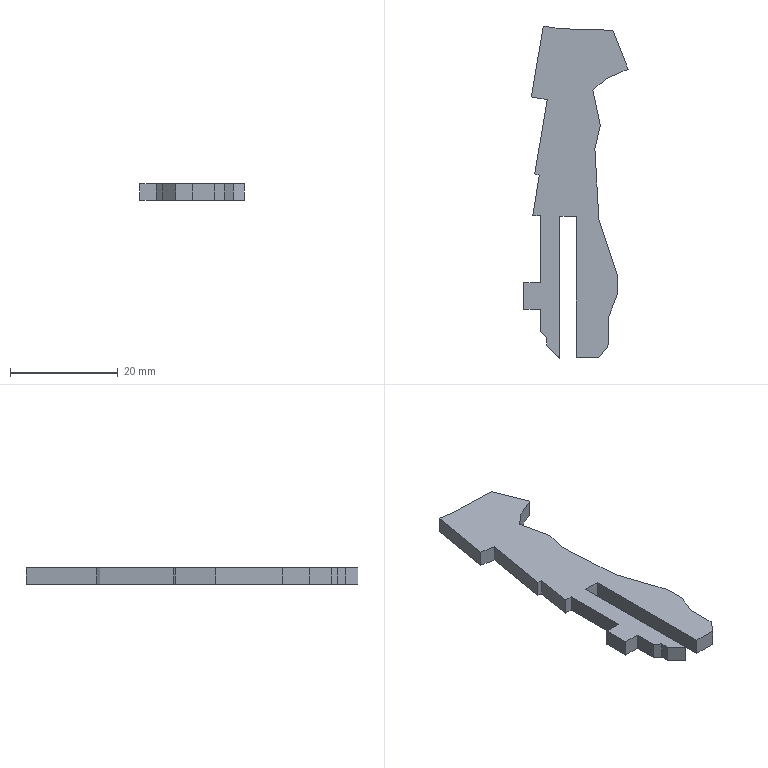Part | SolidWorks | features BaseBody 1 | 1 solid | 33 faces | box 19.346 x 61.524 x 3 mm | volume 2044 mm3 | spline 18 | plane 15
STEP:
#1=CARTESIAN_POINT('',(30.02,-31.07,-1.5));
#2=VERTEX_POINT('',#1);
#3=CARTESIAN_POINT('',(29.997,-32.532,-1.5));
#4=VERTEX_POINT('',#3);
#5=CARTESIAN_POINT('',(30.02,-31.07,-1.5));
#6=CARTESIAN_POINT('',(30.011,-31.556,-1.5));
#7=CARTESIAN_POINT('',(30.004,-32.045,-1.5));
#8=CARTESIAN_POINT('',(29.997,-32.532,-1.5));
#9=B_SPLINE_CURVE_WITH_KNOTS('',3,(#5,#6,#7,#8),.UNSPECIFIED.,.F.,.F.,(4,4),(0.,0.02857),.UNSPECIFIED.);
#10=EDGE_CURVE('',#2,#4,#9,.T.);
#11=ORIENTED_EDGE('',*,*,#10,.F.);
#12=CARTESIAN_POINT('',(28.815,-30.046,-1.5));
#13=VERTEX_POINT('',#12);
#14=CARTESIAN_POINT('',(28.815,-30.046,-1.5));
#15=CARTESIAN_POINT('',(29.216,-30.385,-1.5));
#16=CARTESIAN_POINT('',(29.619,-30.728,-1.5));
#17=CARTESIAN_POINT('',(30.02,-31.07,-1.5));
#18=B_SPLINE_CURVE_WITH_KNOTS('',3,(#14,#15,#16,#17),.UNSPECIFIED.,.F.,.F.,(4,4),(0.02857,0.05714),.UNSPECIFIED.);
#19=EDGE_CURVE('',#13,#2,#18,.T.);
#20=ORIENTED_EDGE('',*,*,#19,.F.);
#21=CARTESIAN_POINT('',(28.813,-25.837,-1.5));
#22=VERTEX_POINT('',#21);
#23=CARTESIAN_POINT('',(28.815,-30.046,-1.5));
#24=DIRECTION('',(0.0006257,-1.,0.));
#25=VECTOR('',#24,1000.);
#26=LINE('',#23,#25);
#27=EDGE_CURVE('',#22,#13,#26,.T.);
#28=ORIENTED_EDGE('',*,*,#27,.F.);
#29=CARTESIAN_POINT('',(25.744,-25.837,-1.5));
#30=VERTEX_POINT('',#29);
#31=CARTESIAN_POINT('',(28.813,-25.837,-1.5));
#32=DIRECTION('',(1.,0.,0.));
#33=VECTOR('',#32,1000.);
#34=LINE('',#31,#33);
#35=EDGE_CURVE('',#30,#22,#34,.T.);
#36=ORIENTED_EDGE('',*,*,#35,.F.);
#37=CARTESIAN_POINT('',(25.744,-20.948,-1.5));
#38=VERTEX_POINT('',#37);
#39=CARTESIAN_POINT('',(25.744,-20.948,-1.5));
#40=DIRECTION('',(0.,-1.,0.));
#41=VECTOR('',#40,1000.);
#42=LINE('',#39,#41);
#43=EDGE_CURVE('',#38,#30,#42,.T.);
#44=ORIENTED_EDGE('',*,*,#43,.F.);
#45=CARTESIAN_POINT('',(28.815,-20.948,-1.5));
#46=VERTEX_POINT('',#45);
#47=CARTESIAN_POINT('',(28.815,-20.948,-1.5));
#48=DIRECTION('',(-1.,0.,0.));
#49=VECTOR('',#48,1000.);
#50=LINE('',#47,#49);
#51=EDGE_CURVE('',#46,#38,#50,.T.);
#52=ORIENTED_EDGE('',*,*,#51,.F.);
#53=CARTESIAN_POINT('',(28.778,-8.507,-1.5));
#54=VERTEX_POINT('',#53);
#55=CARTESIAN_POINT('',(28.778,-8.507,-1.5));
#56=DIRECTION('',(0.00303,-1.,0.));
#57=VECTOR('',#56,1000.);
#58=LINE('',#55,#57);
#59=EDGE_CURVE('',#54,#46,#58,.T.);
#60=ORIENTED_EDGE('',*,*,#59,.F.);
#61=CARTESIAN_POINT('',(27.416,-8.51,-1.5));
#62=VERTEX_POINT('',#61);
#63=CARTESIAN_POINT('',(27.416,-8.51,-1.5));
#64=DIRECTION('',(1.,0.002423,0.));
#65=VECTOR('',#64,1000.);
#66=LINE('',#63,#65);
#67=EDGE_CURVE('',#62,#54,#66,.T.);
#68=ORIENTED_EDGE('',*,*,#67,.F.);
#69=CARTESIAN_POINT('',(28.599,-0.9958,-1.5));
#70=VERTEX_POINT('',#69);
#71=CARTESIAN_POINT('',(28.599,-0.9958,-1.5));
#72=DIRECTION('',(-0.1555,-0.9878,0.));
#73=VECTOR('',#72,1000.);
#74=LINE('',#71,#73);
#75=EDGE_CURVE('',#70,#62,#74,.T.);
#76=ORIENTED_EDGE('',*,*,#75,.F.);
#77=CARTESIAN_POINT('',(27.774,-0.7876,-1.5));
#78=VERTEX_POINT('',#77);
#79=CARTESIAN_POINT('',(27.774,-0.7876,-1.5));
#80=CARTESIAN_POINT('',(28.05,-0.8589,-1.5));
#81=CARTESIAN_POINT('',(28.599,-0.9958,-1.5));
#82=B_SPLINE_CURVE_WITH_KNOTS('',2,(#79,#80,#81),.UNSPECIFIED.,.F.,.F.,(3,3),(0.3143,0.3429),.UNSPECIFIED.);
#83=EDGE_CURVE('',#78,#70,#82,.T.);
#84=ORIENTED_EDGE('',*,*,#83,.F.);
#85=CARTESIAN_POINT('',(30.092,12.981,-1.5));
#86=VERTEX_POINT('',#85);
#87=CARTESIAN_POINT('',(30.092,12.981,-1.5));
#88=CARTESIAN_POINT('',(29.321,8.39,-1.5));
#89=CARTESIAN_POINT('',(28.549,3.8,-1.5));
#90=CARTESIAN_POINT('',(27.774,-0.7876,-1.5));
#91=B_SPLINE_CURVE_WITH_KNOTS('',3,(#87,#88,#89,#90),.UNSPECIFIED.,.F.,.F.,(4,4),(0.3429,0.3714),.UNSPECIFIED.);
#92=EDGE_CURVE('',#86,#78,#91,.T.);
#93=ORIENTED_EDGE('',*,*,#92,.F.);
#94=CARTESIAN_POINT('',(27.138,13.478,-1.5));
#95=VERTEX_POINT('',#94);
#96=CARTESIAN_POINT('',(30.092,12.981,-1.5));
#97=DIRECTION('',(0.9861,-0.1659,0.));
#98=VECTOR('',#97,1000.);
#99=LINE('',#96,#98);
#100=EDGE_CURVE('',#95,#86,#99,.T.);
#101=ORIENTED_EDGE('',*,*,#100,.F.);
#102=CARTESIAN_POINT('',(29.351,26.625,-1.5));
#103=VERTEX_POINT('',#102);
#104=CARTESIAN_POINT('',(29.351,26.625,-1.5));
#105=CARTESIAN_POINT('',(28.613,22.242,-1.5));
#106=CARTESIAN_POINT('',(27.876,17.86,-1.5));
#107=CARTESIAN_POINT('',(27.138,13.478,-1.5));
#108=B_SPLINE_CURVE_WITH_KNOTS('',3,(#104,#105,#106,#107),.UNSPECIFIED.,.F.,.F.,(4,4),(0.4,0.4286),.UNSPECIFIED.);
#109=EDGE_CURVE('',#103,#95,#108,.T.);
#110=ORIENTED_EDGE('',*,*,#109,.F.);
#111=CARTESIAN_POINT('',(32.305,26.126,-1.5));
#112=VERTEX_POINT('',#111);
#113=CARTESIAN_POINT('',(32.305,26.126,-1.5));
#114=CARTESIAN_POINT('',(31.321,26.292,-1.5));
#115=CARTESIAN_POINT('',(30.333,26.457,-1.5));
#116=CARTESIAN_POINT('',(29.351,26.625,-1.5));
#117=B_SPLINE_CURVE_WITH_KNOTS('',3,(#113,#114,#115,#116),.UNSPECIFIED.,.F.,.F.,(4,4),(0.4286,0.4571),.UNSPECIFIED.);
#118=EDGE_CURVE('',#112,#103,#117,.T.);
#119=ORIENTED_EDGE('',*,*,#118,.F.);
#120=CARTESIAN_POINT('',(42.267,25.835,-1.5));
#121=VERTEX_POINT('',#120);
#122=CARTESIAN_POINT('',(42.267,25.835,-1.5));
#123=CARTESIAN_POINT('',(38.946,25.932,-1.5));
#124=CARTESIAN_POINT('',(35.626,26.029,-1.5));
#125=CARTESIAN_POINT('',(32.305,26.126,-1.5));
#126=B_SPLINE_CURVE_WITH_KNOTS('',3,(#122,#123,#124,#125),.UNSPECIFIED.,.F.,.F.,(4,4),(0.4571,0.4857),.UNSPECIFIED.);
#127=EDGE_CURVE('',#121,#112,#126,.T.);
#128=ORIENTED_EDGE('',*,*,#127,.F.);
#129=CARTESIAN_POINT('',(45.09,18.64,-1.5));
#130=VERTEX_POINT('',#129);
#131=CARTESIAN_POINT('',(45.09,18.64,-1.5));
#132=CARTESIAN_POINT('',(44.147,21.036,-1.5));
#133=CARTESIAN_POINT('',(43.208,23.437,-1.5));
#134=CARTESIAN_POINT('',(42.267,25.835,-1.5));
#135=B_SPLINE_CURVE_WITH_KNOTS('',3,(#131,#132,#133,#134),.UNSPECIFIED.,.F.,.F.,(4,4),(0.4857,0.5143),.UNSPECIFIED.);
#136=EDGE_CURVE('',#130,#121,#135,.T.);
#137=ORIENTED_EDGE('',*,*,#136,.F.);
#138=CARTESIAN_POINT('',(41.02,16.861,-1.5));
#139=VERTEX_POINT('',#138);
#140=CARTESIAN_POINT('',(41.02,16.861,-1.5));
#141=CARTESIAN_POINT('',(42.375,17.453,-1.5));
#142=CARTESIAN_POINT('',(43.731,18.045,-1.5));
#143=CARTESIAN_POINT('',(45.09,18.64,-1.5));
#144=B_SPLINE_CURVE_WITH_KNOTS('',3,(#140,#141,#142,#143),.UNSPECIFIED.,.F.,.F.,(4,4),(0.5143,0.5429),.UNSPECIFIED.);
#145=EDGE_CURVE('',#139,#130,#144,.T.);
#146=ORIENTED_EDGE('',*,*,#145,.F.);
#147=CARTESIAN_POINT('',(38.537,14.762,-1.5));
#148=VERTEX_POINT('',#147);
#149=CARTESIAN_POINT('',(38.537,14.762,-1.5));
#150=CARTESIAN_POINT('',(39.365,15.462,-1.5));
#151=CARTESIAN_POINT('',(40.192,16.16,-1.5));
#152=CARTESIAN_POINT('',(41.02,16.861,-1.5));
#153=B_SPLINE_CURVE_WITH_KNOTS('',3,(#149,#150,#151,#152),.UNSPECIFIED.,.F.,.F.,(4,4),(0.5429,0.5714),.UNSPECIFIED.);
#154=EDGE_CURVE('',#148,#139,#153,.T.);
#155=ORIENTED_EDGE('',*,*,#154,.F.);
#156=CARTESIAN_POINT('',(39.944,8.225,-1.5));
#157=VERTEX_POINT('',#156);
#158=CARTESIAN_POINT('',(39.944,8.225,-1.5));
#159=CARTESIAN_POINT('',(39.476,10.405,-1.5));
#160=CARTESIAN_POINT('',(39.007,12.583,-1.5));
#161=CARTESIAN_POINT('',(38.537,14.762,-1.5));
#162=B_SPLINE_CURVE_WITH_KNOTS('',3,(#158,#159,#160,#161),.UNSPECIFIED.,.F.,.F.,(4,4),(0.5714,0.6),.UNSPECIFIED.);
#163=EDGE_CURVE('',#157,#148,#162,.T.);
#164=ORIENTED_EDGE('',*,*,#163,.F.);
#165=CARTESIAN_POINT('',(38.908,3.871,-1.5));
#166=VERTEX_POINT('',#165);
#167=CARTESIAN_POINT('',(38.908,3.871,-1.5));
#168=CARTESIAN_POINT('',(39.252,5.323,-1.5));
#169=CARTESIAN_POINT('',(39.599,6.773,-1.5));
#170=CARTESIAN_POINT('',(39.944,8.225,-1.5));
#171=B_SPLINE_CURVE_WITH_KNOTS('',3,(#167,#168,#169,#170),.UNSPECIFIED.,.F.,.F.,(4,4),(0.6,0.6286),.UNSPECIFIED.);
#172=EDGE_CURVE('',#166,#157,#171,.T.);
#173=ORIENTED_EDGE('',*,*,#172,.F.);
#174=CARTESIAN_POINT('',(39.663,-9.187,-1.5));
#175=VERTEX_POINT('',#174);
#176=CARTESIAN_POINT('',(39.663,-9.187,-1.5));
#177=CARTESIAN_POINT('',(39.412,-4.833,-1.5));
#178=CARTESIAN_POINT('',(39.161,-0.4812,-1.5));
#179=CARTESIAN_POINT('',(38.908,3.871,-1.5));
#180=B_SPLINE_CURVE_WITH_KNOTS('',3,(#176,#177,#178,#179),.UNSPECIFIED.,.F.,.F.,(4,4),(0.6286,0.6571),.UNSPECIFIED.);
#181=EDGE_CURVE('',#175,#166,#180,.T.);
#182=ORIENTED_EDGE('',*,*,#181,.F.);
#183=CARTESIAN_POINT('',(43.061,-19.404,-1.5));
#184=VERTEX_POINT('',#183);
#185=CARTESIAN_POINT('',(43.061,-19.404,-1.5));
#186=CARTESIAN_POINT('',(41.93,-15.998,-1.5));
#187=CARTESIAN_POINT('',(40.796,-12.592,-1.5));
#188=CARTESIAN_POINT('',(39.663,-9.187,-1.5));
#189=B_SPLINE_CURVE_WITH_KNOTS('',3,(#185,#186,#187,#188),.UNSPECIFIED.,.F.,.F.,(4,4),(0.6571,0.6857),.UNSPECIFIED.);
#190=EDGE_CURVE('',#184,#175,#189,.T.);
#191=ORIENTED_EDGE('',*,*,#190,.F.);
#192=CARTESIAN_POINT('',(43.089,-23.124,-1.5));
#193=VERTEX_POINT('',#192);
#194=CARTESIAN_POINT('',(43.089,-23.124,-1.5));
#195=CARTESIAN_POINT('',(43.078,-21.885,-1.5));
#196=CARTESIAN_POINT('',(43.071,-20.645,-1.5));
#197=CARTESIAN_POINT('',(43.061,-19.404,-1.5));
#198=B_SPLINE_CURVE_WITH_KNOTS('',3,(#194,#195,#196,#197),.UNSPECIFIED.,.F.,.F.,(4,4),(0.6857,0.7143),.UNSPECIFIED.);
#199=EDGE_CURVE('',#193,#184,#198,.T.);
#200=ORIENTED_EDGE('',*,*,#199,.F.);
#201=CARTESIAN_POINT('',(41.448,-27.362,-1.5));
#202=VERTEX_POINT('',#201);
#203=CARTESIAN_POINT('',(41.448,-27.362,-1.5));
#204=CARTESIAN_POINT('',(41.993,-25.948,-1.5));
#205=CARTESIAN_POINT('',(42.541,-24.536,-1.5));
#206=CARTESIAN_POINT('',(43.089,-23.124,-1.5));
#207=B_SPLINE_CURVE_WITH_KNOTS('',3,(#203,#204,#205,#206),.UNSPECIFIED.,.F.,.F.,(4,4),(0.7143,0.7429),.UNSPECIFIED.);
#208=EDGE_CURVE('',#202,#193,#207,.T.);
#209=ORIENTED_EDGE('',*,*,#208,.F.);
#210=CARTESIAN_POINT('',(41.486,-32.484,-1.5));
#211=VERTEX_POINT('',#210);
#212=CARTESIAN_POINT('',(41.486,-32.484,-1.5));
#213=CARTESIAN_POINT('',(41.472,-30.775,-1.5));
#214=CARTESIAN_POINT('',(41.46,-29.068,-1.5));
#215=CARTESIAN_POINT('',(41.448,-27.362,-1.5));
#216=B_SPLINE_CURVE_WITH_KNOTS('',3,(#212,#213,#214,#215),.UNSPECIFIED.,.F.,.F.,(4,4),(0.7429,0.7714),.UNSPECIFIED.);
#217=EDGE_CURVE('',#211,#202,#216,.T.);
#218=ORIENTED_EDGE('',*,*,#217,.F.);
#219=CARTESIAN_POINT('',(39.634,-34.791,-1.5));
#220=VERTEX_POINT('',#219);
#221=CARTESIAN_POINT('',(39.634,-34.791,-1.5));
#222=CARTESIAN_POINT('',(40.25,-34.022,-1.5));
#223=CARTESIAN_POINT('',(40.867,-33.253,-1.5));
#224=CARTESIAN_POINT('',(41.486,-32.484,-1.5));
#225=B_SPLINE_CURVE_WITH_KNOTS('',3,(#221,#222,#223,#224),.UNSPECIFIED.,.F.,.F.,(4,4),(0.7714,0.8),.UNSPECIFIED.);
#226=EDGE_CURVE('',#220,#211,#225,.T.);
#227=ORIENTED_EDGE('',*,*,#226,.F.);
#228=CARTESIAN_POINT('',(35.441,-34.791,-1.5));
#229=VERTEX_POINT('',#228);
#230=CARTESIAN_POINT('',(39.634,-34.791,-1.5));
#231=DIRECTION('',(1.,0.,0.));
#232=VECTOR('',#231,1000.);
#233=LINE('',#230,#232);
#234=EDGE_CURVE('',#229,#220,#233,.T.);
#235=ORIENTED_EDGE('',*,*,#234,.F.);
#236=CARTESIAN_POINT('',(35.441,-8.666,-1.5));
#237=VERTEX_POINT('',#236);
#238=CARTESIAN_POINT('',(35.441,-34.791,-1.5));
#239=DIRECTION('',(0.,-1.,0.));
#240=VECTOR('',#239,1000.);
#241=LINE('',#238,#240);
#242=EDGE_CURVE('',#237,#229,#241,.T.);
#243=ORIENTED_EDGE('',*,*,#242,.F.);
#244=CARTESIAN_POINT('',(32.445,-8.666,-1.5));
#245=VERTEX_POINT('',#244);
#246=CARTESIAN_POINT('',(35.441,-8.666,-1.5));
#247=DIRECTION('',(1.,0.000000244,0.));
#248=VECTOR('',#247,1000.);
#249=LINE('',#246,#248);
#250=EDGE_CURVE('',#245,#237,#249,.T.);
#251=ORIENTED_EDGE('',*,*,#250,.F.);
#252=CARTESIAN_POINT('',(32.445,-34.899,-1.5));
#253=VERTEX_POINT('',#252);
#254=CARTESIAN_POINT('',(32.445,-8.666,-1.5));
#255=DIRECTION('',(0.,1.,0.));
#256=VECTOR('',#255,1000.);
#257=LINE('',#254,#256);
#258=EDGE_CURVE('',#253,#245,#257,.T.);
#259=ORIENTED_EDGE('',*,*,#258,.F.);
#260=CARTESIAN_POINT('',(32.445,-34.899,-1.5));
#261=DIRECTION('',(0.7188,-0.6952,0.));
#262=VECTOR('',#261,1000.);
#263=LINE('',#260,#262);
#264=EDGE_CURVE('',#4,#253,#263,.T.);
#265=ORIENTED_EDGE('',*,*,#264,.F.);
#266=EDGE_LOOP('',(#11,#20,#28,#36,#44,#52,#60,#68,#76,#84,#93,#101,#110,#119,#128,#137,#146,#155,#164,#173,#182,#191,#200,#209,#218,#227,#235,#243,#251,#259,#265));
#267=FACE_OUTER_BOUND('',#266,.T.);
#268=CARTESIAN_POINT('',(30.008,-31.801,-1.5));
#269=DIRECTION('',(0.,0.,1.));
#270=DIRECTION('',(1.,0.,0.));
#271=AXIS2_PLACEMENT_3D('',#268,#269,#270);
#272=PLANE('',#271);
#273=ADVANCED_FACE('',(#267),#272,.F.);
#274=CARTESIAN_POINT('',(30.02,-31.07,1.5));
#275=VERTEX_POINT('',#274);
#276=CARTESIAN_POINT('',(29.997,-32.532,1.5));
#277=VERTEX_POINT('',#276);
#278=CARTESIAN_POINT('',(30.02,-31.07,1.5));
#279=CARTESIAN_POINT('',(30.011,-31.556,1.5));
#280=CARTESIAN_POINT('',(30.004,-32.045,1.5));
#281=CARTESIAN_POINT('',(29.997,-32.532,1.5));
#282=B_SPLINE_CURVE_WITH_KNOTS('',3,(#278,#279,#280,#281),.UNSPECIFIED.,.F.,.F.,(4,4),(0.,0.02857),.UNSPECIFIED.);
#283=EDGE_CURVE('',#275,#277,#282,.T.);
#284=ORIENTED_EDGE('',*,*,#283,.T.);
#285=CARTESIAN_POINT('',(32.445,-34.899,1.5));
#286=VERTEX_POINT('',#285);
#287=CARTESIAN_POINT('',(32.445,-34.899,1.5));
#288=DIRECTION('',(0.7188,-0.6952,0.));
#289=VECTOR('',#288,1000.);
#290=LINE('',#287,#289);
#291=EDGE_CURVE('',#277,#286,#290,.T.);
#292=ORIENTED_EDGE('',*,*,#291,.T.);
#293=CARTESIAN_POINT('',(32.445,-8.666,1.5));
#294=VERTEX_POINT('',#293);
#295=CARTESIAN_POINT('',(32.445,-8.666,1.5));
#296=DIRECTION('',(0.,1.,0.));
#297=VECTOR('',#296,1000.);
#298=LINE('',#295,#297);
#299=EDGE_CURVE('',#286,#294,#298,.T.);
#300=ORIENTED_EDGE('',*,*,#299,.T.);
#301=CARTESIAN_POINT('',(35.441,-8.666,1.5));
#302=VERTEX_POINT('',#301);
#303=CARTESIAN_POINT('',(35.441,-8.666,1.5));
#304=DIRECTION('',(1.,0.000000244,0.));
#305=VECTOR('',#304,1000.);
#306=LINE('',#303,#305);
#307=EDGE_CURVE('',#294,#302,#306,.T.);
#308=ORIENTED_EDGE('',*,*,#307,.T.);
#309=CARTESIAN_POINT('',(35.441,-34.791,1.5));
#310=VERTEX_POINT('',#309);
#311=CARTESIAN_POINT('',(35.441,-34.791,1.5));
#312=DIRECTION('',(0.,-1.,0.));
#313=VECTOR('',#312,1000.);
#314=LINE('',#311,#313);
#315=EDGE_CURVE('',#302,#310,#314,.T.);
#316=ORIENTED_EDGE('',*,*,#315,.T.);
#317=CARTESIAN_POINT('',(39.634,-34.791,1.5));
#318=VERTEX_POINT('',#317);
#319=CARTESIAN_POINT('',(39.634,-34.791,1.5));
#320=DIRECTION('',(1.,0.,0.));
#321=VECTOR('',#320,1000.);
#322=LINE('',#319,#321);
#323=EDGE_CURVE('',#310,#318,#322,.T.);
#324=ORIENTED_EDGE('',*,*,#323,.T.);
#325=CARTESIAN_POINT('',(41.486,-32.484,1.5));
#326=VERTEX_POINT('',#325);
#327=CARTESIAN_POINT('',(39.634,-34.791,1.5));
#328=CARTESIAN_POINT('',(40.25,-34.022,1.5));
#329=CARTESIAN_POINT('',(40.867,-33.253,1.5));
#330=CARTESIAN_POINT('',(41.486,-32.484,1.5));
#331=B_SPLINE_CURVE_WITH_KNOTS('',3,(#327,#328,#329,#330),.UNSPECIFIED.,.F.,.F.,(4,4),(0.7714,0.8),.UNSPECIFIED.);
#332=EDGE_CURVE('',#318,#326,#331,.T.);
#333=ORIENTED_EDGE('',*,*,#332,.T.);
#334=CARTESIAN_POINT('',(41.448,-27.362,1.5));
#335=VERTEX_POINT('',#334);
#336=CARTESIAN_POINT('',(41.486,-32.484,1.5));
#337=CARTESIAN_POINT('',(41.472,-30.775,1.5));
#338=CARTESIAN_POINT('',(41.46,-29.068,1.5));
#339=CARTESIAN_POINT('',(41.448,-27.362,1.5));
#340=B_SPLINE_CURVE_WITH_KNOTS('',3,(#336,#337,#338,#339),.UNSPECIFIED.,.F.,.F.,(4,4),(0.7429,0.7714),.UNSPECIFIED.);
#341=EDGE_CURVE('',#326,#335,#340,.T.);
#342=ORIENTED_EDGE('',*,*,#341,.T.);
#343=CARTESIAN_POINT('',(43.089,-23.124,1.5));
#344=VERTEX_POINT('',#343);
#345=CARTESIAN_POINT('',(41.448,-27.362,1.5));
#346=CARTESIAN_POINT('',(41.993,-25.948,1.5));
#347=CARTESIAN_POINT('',(42.541,-24.536,1.5));
#348=CARTESIAN_POINT('',(43.089,-23.124,1.5));
#349=B_SPLINE_CURVE_WITH_KNOTS('',3,(#345,#346,#347,#348),.UNSPECIFIED.,.F.,.F.,(4,4),(0.7143,0.7429),.UNSPECIFIED.);
#350=EDGE_CURVE('',#335,#344,#349,.T.);
#351=ORIENTED_EDGE('',*,*,#350,.T.);
#352=CARTESIAN_POINT('',(43.061,-19.404,1.5));
#353=VERTEX_POINT('',#352);
#354=CARTESIAN_POINT('',(43.089,-23.124,1.5));
#355=CARTESIAN_POINT('',(43.078,-21.885,1.5));
#356=CARTESIAN_POINT('',(43.071,-20.645,1.5));
#357=CARTESIAN_POINT('',(43.061,-19.404,1.5));
#358=B_SPLINE_CURVE_WITH_KNOTS('',3,(#354,#355,#356,#357),.UNSPECIFIED.,.F.,.F.,(4,4),(0.6857,0.7143),.UNSPECIFIED.);
#359=EDGE_CURVE('',#344,#353,#358,.T.);
#360=ORIENTED_EDGE('',*,*,#359,.T.);
#361=CARTESIAN_POINT('',(39.663,-9.187,1.5));
#362=VERTEX_POINT('',#361);
#363=CARTESIAN_POINT('',(43.061,-19.404,1.5));
#364=CARTESIAN_POINT('',(41.93,-15.998,1.5));
#365=CARTESIAN_POINT('',(40.796,-12.592,1.5));
#366=CARTESIAN_POINT('',(39.663,-9.187,1.5));
#367=B_SPLINE_CURVE_WITH_KNOTS('',3,(#363,#364,#365,#366),.UNSPECIFIED.,.F.,.F.,(4,4),(0.6571,0.6857),.UNSPECIFIED.);
#368=EDGE_CURVE('',#353,#362,#367,.T.);
#369=ORIENTED_EDGE('',*,*,#368,.T.);
#370=CARTESIAN_POINT('',(38.908,3.871,1.5));
#371=VERTEX_POINT('',#370);
#372=CARTESIAN_POINT('',(39.663,-9.187,1.5));
#373=CARTESIAN_POINT('',(39.412,-4.833,1.5));
#374=CARTESIAN_POINT('',(39.161,-0.4812,1.5));
#375=CARTESIAN_POINT('',(38.908,3.871,1.5));
#376=B_SPLINE_CURVE_WITH_KNOTS('',3,(#372,#373,#374,#375),.UNSPECIFIED.,.F.,.F.,(4,4),(0.6286,0.6571),.UNSPECIFIED.);
#377=EDGE_CURVE('',#362,#371,#376,.T.);
#378=ORIENTED_EDGE('',*,*,#377,.T.);
#379=CARTESIAN_POINT('',(39.944,8.225,1.5));
#380=VERTEX_POINT('',#379);
#381=CARTESIAN_POINT('',(38.908,3.871,1.5));
#382=CARTESIAN_POINT('',(39.252,5.323,1.5));
#383=CARTESIAN_POINT('',(39.599,6.773,1.5));
#384=CARTESIAN_POINT('',(39.944,8.225,1.5));
#385=B_SPLINE_CURVE_WITH_KNOTS('',3,(#381,#382,#383,#384),.UNSPECIFIED.,.F.,.F.,(4,4),(0.6,0.6286),.UNSPECIFIED.);
#386=EDGE_CURVE('',#371,#380,#385,.T.);
#387=ORIENTED_EDGE('',*,*,#386,.T.);
#388=CARTESIAN_POINT('',(38.537,14.762,1.5));
#389=VERTEX_POINT('',#388);
#390=CARTESIAN_POINT('',(39.944,8.225,1.5));
#391=CARTESIAN_POINT('',(39.476,10.405,1.5));
#392=CARTESIAN_POINT('',(39.007,12.583,1.5));
#393=CARTESIAN_POINT('',(38.537,14.762,1.5));
#394=B_SPLINE_CURVE_WITH_KNOTS('',3,(#390,#391,#392,#393),.UNSPECIFIED.,.F.,.F.,(4,4),(0.5714,0.6),.UNSPECIFIED.);
#395=EDGE_CURVE('',#380,#389,#394,.T.);
#396=ORIENTED_EDGE('',*,*,#395,.T.);
#397=CARTESIAN_POINT('',(41.02,16.861,1.5));
#398=VERTEX_POINT('',#397);
#399=CARTESIAN_POINT('',(38.537,14.762,1.5));
#400=CARTESIAN_POINT('',(39.365,15.462,1.5));
#401=CARTESIAN_POINT('',(40.192,16.16,1.5));
#402=CARTESIAN_POINT('',(41.02,16.861,1.5));
#403=B_SPLINE_CURVE_WITH_KNOTS('',3,(#399,#400,#401,#402),.UNSPECIFIED.,.F.,.F.,(4,4),(0.5429,0.5714),.UNSPECIFIED.);
#404=EDGE_CURVE('',#389,#398,#403,.T.);
#405=ORIENTED_EDGE('',*,*,#404,.T.);
#406=CARTESIAN_POINT('',(45.09,18.64,1.5));
#407=VERTEX_POINT('',#406);
#408=CARTESIAN_POINT('',(41.02,16.861,1.5));
#409=CARTESIAN_POINT('',(42.375,17.453,1.5));
#410=CARTESIAN_POINT('',(43.731,18.045,1.5));
#411=CARTESIAN_POINT('',(45.09,18.64,1.5));
#412=B_SPLINE_CURVE_WITH_KNOTS('',3,(#408,#409,#410,#411),.UNSPECIFIED.,.F.,.F.,(4,4),(0.5143,0.5429),.UNSPECIFIED.);
#413=EDGE_CURVE('',#398,#407,#412,.T.);
#414=ORIENTED_EDGE('',*,*,#413,.T.);
#415=CARTESIAN_POINT('',(42.267,25.835,1.5));
#416=VERTEX_POINT('',#415);
#417=CARTESIAN_POINT('',(45.09,18.64,1.5));
#418=CARTESIAN_POINT('',(44.147,21.036,1.5));
#419=CARTESIAN_POINT('',(43.208,23.437,1.5));
#420=CARTESIAN_POINT('',(42.267,25.835,1.5));
#421=B_SPLINE_CURVE_WITH_KNOTS('',3,(#417,#418,#419,#420),.UNSPECIFIED.,.F.,.F.,(4,4),(0.4857,0.5143),.UNSPECIFIED.);
#422=EDGE_CURVE('',#407,#416,#421,.T.);
#423=ORIENTED_EDGE('',*,*,#422,.T.);
#424=CARTESIAN_POINT('',(32.305,26.126,1.5));
#425=VERTEX_POINT('',#424);
#426=CARTESIAN_POINT('',(42.267,25.835,1.5));
#427=CARTESIAN_POINT('',(38.946,25.932,1.5));
#428=CARTESIAN_POINT('',(35.626,26.029,1.5));
#429=CARTESIAN_POINT('',(32.305,26.126,1.5));
#430=B_SPLINE_CURVE_WITH_KNOTS('',3,(#426,#427,#428,#429),.UNSPECIFIED.,.F.,.F.,(4,4),(0.4571,0.4857),.UNSPECIFIED.);
#431=EDGE_CURVE('',#416,#425,#430,.T.);
#432=ORIENTED_EDGE('',*,*,#431,.T.);
#433=CARTESIAN_POINT('',(29.351,26.625,1.5));
#434=VERTEX_POINT('',#433);
#435=CARTESIAN_POINT('',(32.305,26.126,1.5));
#436=CARTESIAN_POINT('',(31.321,26.292,1.5));
#437=CARTESIAN_POINT('',(30.333,26.457,1.5));
#438=CARTESIAN_POINT('',(29.351,26.625,1.5));
#439=B_SPLINE_CURVE_WITH_KNOTS('',3,(#435,#436,#437,#438),.UNSPECIFIED.,.F.,.F.,(4,4),(0.4286,0.4571),.UNSPECIFIED.);
#440=EDGE_CURVE('',#425,#434,#439,.T.);
#441=ORIENTED_EDGE('',*,*,#440,.T.);
#442=CARTESIAN_POINT('',(27.138,13.478,1.5));
#443=VERTEX_POINT('',#442);
#444=CARTESIAN_POINT('',(29.351,26.625,1.5));
#445=CARTESIAN_POINT('',(28.613,22.242,1.5));
#446=CARTESIAN_POINT('',(27.876,17.86,1.5));
#447=CARTESIAN_POINT('',(27.138,13.478,1.5));
#448=B_SPLINE_CURVE_WITH_KNOTS('',3,(#444,#445,#446,#447),.UNSPECIFIED.,.F.,.F.,(4,4),(0.4,0.4286),.UNSPECIFIED.);
#449=EDGE_CURVE('',#434,#443,#448,.T.);
#450=ORIENTED_EDGE('',*,*,#449,.T.);
#451=CARTESIAN_POINT('',(30.092,12.981,1.5));
#452=VERTEX_POINT('',#451);
#453=CARTESIAN_POINT('',(30.092,12.981,1.5));
#454=DIRECTION('',(0.9861,-0.1659,0.));
#455=VECTOR('',#454,1000.);
#456=LINE('',#453,#455);
#457=EDGE_CURVE('',#443,#452,#456,.T.);
#458=ORIENTED_EDGE('',*,*,#457,.T.);
#459=CARTESIAN_POINT('',(27.774,-0.7876,1.5));
#460=VERTEX_POINT('',#459);
#461=CARTESIAN_POINT('',(30.092,12.981,1.5));
#462=CARTESIAN_POINT('',(29.321,8.39,1.5));
#463=CARTESIAN_POINT('',(28.549,3.8,1.5));
#464=CARTESIAN_POINT('',(27.774,-0.7876,1.5));
#465=B_SPLINE_CURVE_WITH_KNOTS('',3,(#461,#462,#463,#464),.UNSPECIFIED.,.F.,.F.,(4,4),(0.3429,0.3714),.UNSPECIFIED.);
#466=EDGE_CURVE('',#452,#460,#465,.T.);
#467=ORIENTED_EDGE('',*,*,#466,.T.);
#468=CARTESIAN_POINT('',(28.599,-0.9958,1.5));
#469=VERTEX_POINT('',#468);
#470=CARTESIAN_POINT('',(27.774,-0.7876,1.5));
#471=CARTESIAN_POINT('',(28.05,-0.8589,1.5));
#472=CARTESIAN_POINT('',(28.599,-0.9958,1.5));
#473=B_SPLINE_CURVE_WITH_KNOTS('',2,(#470,#471,#472),.UNSPECIFIED.,.F.,.F.,(3,3),(0.3143,0.3429),.UNSPECIFIED.);
#474=EDGE_CURVE('',#460,#469,#473,.T.);
#475=ORIENTED_EDGE('',*,*,#474,.T.);
#476=CARTESIAN_POINT('',(27.416,-8.51,1.5));
#477=VERTEX_POINT('',#476);
#478=CARTESIAN_POINT('',(28.599,-0.9958,1.5));
#479=DIRECTION('',(-0.1555,-0.9878,0.));
#480=VECTOR('',#479,1000.);
#481=LINE('',#478,#480);
#482=EDGE_CURVE('',#469,#477,#481,.T.);
#483=ORIENTED_EDGE('',*,*,#482,.T.);
#484=CARTESIAN_POINT('',(28.778,-8.507,1.5));
#485=VERTEX_POINT('',#484);
#486=CARTESIAN_POINT('',(27.416,-8.51,1.5));
#487=DIRECTION('',(1.,0.002423,0.));
#488=VECTOR('',#487,1000.);
#489=LINE('',#486,#488);
#490=EDGE_CURVE('',#477,#485,#489,.T.);
#491=ORIENTED_EDGE('',*,*,#490,.T.);
#492=CARTESIAN_POINT('',(28.815,-20.948,1.5));
#493=VERTEX_POINT('',#492);
#494=CARTESIAN_POINT('',(28.778,-8.507,1.5));
#495=DIRECTION('',(0.00303,-1.,0.));
#496=VECTOR('',#495,1000.);
#497=LINE('',#494,#496);
#498=EDGE_CURVE('',#485,#493,#497,.T.);
#499=ORIENTED_EDGE('',*,*,#498,.T.);
#500=CARTESIAN_POINT('',(25.744,-20.948,1.5));
#501=VERTEX_POINT('',#500);
#502=CARTESIAN_POINT('',(28.815,-20.948,1.5));
#503=DIRECTION('',(-1.,0.,0.));
#504=VECTOR('',#503,1000.);
#505=LINE('',#502,#504);
#506=EDGE_CURVE('',#493,#501,#505,.T.);
#507=ORIENTED_EDGE('',*,*,#506,.T.);
#508=CARTESIAN_POINT('',(25.744,-25.837,1.5));
#509=VERTEX_POINT('',#508);
#510=CARTESIAN_POINT('',(25.744,-20.948,1.5));
#511=DIRECTION('',(0.,-1.,0.));
#512=VECTOR('',#511,1000.);
#513=LINE('',#510,#512);
#514=EDGE_CURVE('',#501,#509,#513,.T.);
#515=ORIENTED_EDGE('',*,*,#514,.T.);
#516=CARTESIAN_POINT('',(28.813,-25.837,1.5));
#517=VERTEX_POINT('',#516);
#518=CARTESIAN_POINT('',(28.813,-25.837,1.5));
#519=DIRECTION('',(1.,0.,0.));
#520=VECTOR('',#519,1000.);
#521=LINE('',#518,#520);
#522=EDGE_CURVE('',#509,#517,#521,.T.);
#523=ORIENTED_EDGE('',*,*,#522,.T.);
#524=CARTESIAN_POINT('',(28.815,-30.046,1.5));
#525=VERTEX_POINT('',#524);
#526=CARTESIAN_POINT('',(28.815,-30.046,1.5));
#527=DIRECTION('',(0.0006257,-1.,0.));
#528=VECTOR('',#527,1000.);
#529=LINE('',#526,#528);
#530=EDGE_CURVE('',#517,#525,#529,.T.);
#531=ORIENTED_EDGE('',*,*,#530,.T.);
#532=CARTESIAN_POINT('',(28.815,-30.046,1.5));
#533=CARTESIAN_POINT('',(29.216,-30.385,1.5));
#534=CARTESIAN_POINT('',(29.619,-30.728,1.5));
#535=CARTESIAN_POINT('',(30.02,-31.07,1.5));
#536=B_SPLINE_CURVE_WITH_KNOTS('',3,(#532,#533,#534,#535),.UNSPECIFIED.,.F.,.F.,(4,4),(0.02857,0.05714),.UNSPECIFIED.);
#537=EDGE_CURVE('',#525,#275,#536,.T.);
#538=ORIENTED_EDGE('',*,*,#537,.T.);
#539=EDGE_LOOP('',(#284,#292,#300,#308,#316,#324,#333,#342,#351,#360,#369,#378,#387,#396,#405,#414,#423,#432,#441,#450,#458,#467,#475,#483,#491,#499,#507,#515,#523,#531,#538));
#540=FACE_OUTER_BOUND('',#539,.T.);
#541=CARTESIAN_POINT('',(30.008,-31.801,1.5));
#542=DIRECTION('',(0.,0.,1.));
#543=DIRECTION('',(1.,0.,0.));
#544=AXIS2_PLACEMENT_3D('',#541,#542,#543);
#545=PLANE('',#544);
#546=ADVANCED_FACE('',(#540),#545,.T.);
#547=ORIENTED_EDGE('',*,*,#19,.T.);
#548=CARTESIAN_POINT('',(30.02,-31.07,1.5));
#549=DIRECTION('',(0.,0.,-1.));
#550=VECTOR('',#549,1000.);
#551=LINE('',#548,#550);
#552=EDGE_CURVE('',#275,#2,#551,.T.);
#553=ORIENTED_EDGE('',*,*,#552,.F.);
#554=ORIENTED_EDGE('',*,*,#537,.F.);
#555=CARTESIAN_POINT('',(28.815,-30.046,1.5));
#556=DIRECTION('',(0.,0.,-1.));
#557=VECTOR('',#556,1000.);
#558=LINE('',#555,#557);
#559=EDGE_CURVE('',#525,#13,#558,.T.);
#560=ORIENTED_EDGE('',*,*,#559,.T.);
#561=EDGE_LOOP('',(#547,#553,#554,#560));
#562=FACE_OUTER_BOUND('',#561,.T.);
#563=CARTESIAN_POINT('',(28.815,-30.046,1.5));
#564=CARTESIAN_POINT('',(28.815,-30.046,-1.5));
#565=CARTESIAN_POINT('',(29.216,-30.385,1.5));
#566=CARTESIAN_POINT('',(29.216,-30.385,-1.5));
#567=CARTESIAN_POINT('',(29.619,-30.728,1.5));
#568=CARTESIAN_POINT('',(29.619,-30.728,-1.5));
#569=CARTESIAN_POINT('',(30.02,-31.07,1.5));
#570=CARTESIAN_POINT('',(30.02,-31.07,-1.5));
#571=B_SPLINE_SURFACE_WITH_KNOTS('',3,1,((#563,#564),(#565,#566),(#567,#568),(#569,#570)),.UNSPECIFIED.,.F.,.F.,.F.,(4,4),(2,2),(0.02857,0.05714),(0.,1.),.UNSPECIFIED.);
#572=ADVANCED_FACE('',(#562),#571,.F.);
#573=ORIENTED_EDGE('',*,*,#27,.T.);
#574=ORIENTED_EDGE('',*,*,#559,.F.);
#575=ORIENTED_EDGE('',*,*,#530,.F.);
#576=CARTESIAN_POINT('',(28.813,-25.837,1.5));
#577=DIRECTION('',(0.,0.,-1.));
#578=VECTOR('',#577,1000.);
#579=LINE('',#576,#578);
#580=EDGE_CURVE('',#517,#22,#579,.T.);
#581=ORIENTED_EDGE('',*,*,#580,.T.);
#582=EDGE_LOOP('',(#573,#574,#575,#581));
#583=FACE_OUTER_BOUND('',#582,.T.);
#584=CARTESIAN_POINT('',(28.815,-30.046,1.5));
#585=DIRECTION('',(1.,0.0006257,0.));
#586=DIRECTION('',(0.,0.,-1.));
#587=AXIS2_PLACEMENT_3D('',#584,#585,#586);
#588=PLANE('',#587);
#589=ADVANCED_FACE('',(#583),#588,.F.);
#590=ORIENTED_EDGE('',*,*,#35,.T.);
#591=ORIENTED_EDGE('',*,*,#580,.F.);
#592=ORIENTED_EDGE('',*,*,#522,.F.);
#593=CARTESIAN_POINT('',(25.744,-25.837,1.5));
#594=DIRECTION('',(0.,0.,-1.));
#595=VECTOR('',#594,1000.);
#596=LINE('',#593,#595);
#597=EDGE_CURVE('',#509,#30,#596,.T.);
#598=ORIENTED_EDGE('',*,*,#597,.T.);
#599=EDGE_LOOP('',(#590,#591,#592,#598));
#600=FACE_OUTER_BOUND('',#599,.T.);
#601=CARTESIAN_POINT('',(28.813,-25.837,1.5));
#602=DIRECTION('',(0.,1.,0.));
#603=DIRECTION('',(1.,0.,0.));
#604=AXIS2_PLACEMENT_3D('',#601,#602,#603);
#605=PLANE('',#604);
#606=ADVANCED_FACE('',(#600),#605,.F.);
#607=ORIENTED_EDGE('',*,*,#43,.T.);
#608=ORIENTED_EDGE('',*,*,#597,.F.);
#609=ORIENTED_EDGE('',*,*,#514,.F.);
#610=CARTESIAN_POINT('',(25.744,-20.948,1.5));
#611=DIRECTION('',(0.,0.,-1.));
#612=VECTOR('',#611,1000.);
#613=LINE('',#610,#612);
#614=EDGE_CURVE('',#501,#38,#613,.T.);
#615=ORIENTED_EDGE('',*,*,#614,.T.);
#616=EDGE_LOOP('',(#607,#608,#609,#615));
#617=FACE_OUTER_BOUND('',#616,.T.);
#618=CARTESIAN_POINT('',(25.744,-20.948,1.5));
#619=DIRECTION('',(1.,0.,0.));
#620=DIRECTION('',(0.,1.,0.));
#621=AXIS2_PLACEMENT_3D('',#618,#619,#620);
#622=PLANE('',#621);
#623=ADVANCED_FACE('',(#617),#622,.F.);
#624=ORIENTED_EDGE('',*,*,#51,.T.);
#625=ORIENTED_EDGE('',*,*,#614,.F.);
#626=ORIENTED_EDGE('',*,*,#506,.F.);
#627=CARTESIAN_POINT('',(28.815,-20.948,1.5));
#628=DIRECTION('',(0.,0.,-1.));
#629=VECTOR('',#628,1000.);
#630=LINE('',#627,#629);
#631=EDGE_CURVE('',#493,#46,#630,.T.);
#632=ORIENTED_EDGE('',*,*,#631,.T.);
#633=EDGE_LOOP('',(#624,#625,#626,#632));
#634=FACE_OUTER_BOUND('',#633,.T.);
#635=CARTESIAN_POINT('',(28.815,-20.948,1.5));
#636=DIRECTION('',(0.,-1.,0.));
#637=DIRECTION('',(0.,0.,-1.));
#638=AXIS2_PLACEMENT_3D('',#635,#636,#637);
#639=PLANE('',#638);
#640=ADVANCED_FACE('',(#634),#639,.F.);
#641=ORIENTED_EDGE('',*,*,#59,.T.);
#642=ORIENTED_EDGE('',*,*,#631,.F.);
#643=ORIENTED_EDGE('',*,*,#498,.F.);
#644=CARTESIAN_POINT('',(28.778,-8.507,1.5));
#645=DIRECTION('',(0.,0.,-1.));
#646=VECTOR('',#645,1000.);
#647=LINE('',#644,#646);
#648=EDGE_CURVE('',#485,#54,#647,.T.);
#649=ORIENTED_EDGE('',*,*,#648,.T.);
#650=EDGE_LOOP('',(#641,#642,#643,#649));
#651=FACE_OUTER_BOUND('',#650,.T.);
#652=CARTESIAN_POINT('',(28.778,-8.507,1.5));
#653=DIRECTION('',(1.,0.00303,0.));
#654=DIRECTION('',(0.,0.,-1.));
#655=AXIS2_PLACEMENT_3D('',#652,#653,#654);
#656=PLANE('',#655);
#657=ADVANCED_FACE('',(#651),#656,.F.);
#658=ORIENTED_EDGE('',*,*,#67,.T.);
#659=ORIENTED_EDGE('',*,*,#648,.F.);
#660=ORIENTED_EDGE('',*,*,#490,.F.);
#661=CARTESIAN_POINT('',(27.416,-8.51,1.5));
#662=DIRECTION('',(0.,0.,-1.));
#663=VECTOR('',#662,1000.);
#664=LINE('',#661,#663);
#665=EDGE_CURVE('',#477,#62,#664,.T.);
#666=ORIENTED_EDGE('',*,*,#665,.T.);
#667=EDGE_LOOP('',(#658,#659,#660,#666));
#668=FACE_OUTER_BOUND('',#667,.T.);
#669=CARTESIAN_POINT('',(27.416,-8.51,1.5));
#670=DIRECTION('',(-0.002423,1.,0.));
#671=DIRECTION('',(0.,0.,1.));
#672=AXIS2_PLACEMENT_3D('',#669,#670,#671);
#673=PLANE('',#672);
#674=ADVANCED_FACE('',(#668),#673,.F.);
#675=ORIENTED_EDGE('',*,*,#75,.T.);
#676=ORIENTED_EDGE('',*,*,#665,.F.);
#677=ORIENTED_EDGE('',*,*,#482,.F.);
#678=CARTESIAN_POINT('',(28.599,-0.9958,1.5));
#679=DIRECTION('',(0.,0.,-1.));
#680=VECTOR('',#679,1000.);
#681=LINE('',#678,#680);
#682=EDGE_CURVE('',#469,#70,#681,.T.);
#683=ORIENTED_EDGE('',*,*,#682,.T.);
#684=EDGE_LOOP('',(#675,#676,#677,#683));
#685=FACE_OUTER_BOUND('',#684,.T.);
#686=CARTESIAN_POINT('',(28.599,-0.9958,1.5));
#687=DIRECTION('',(0.9878,-0.1555,0.));
#688=DIRECTION('',(0.,0.,-1.));
#689=AXIS2_PLACEMENT_3D('',#686,#687,#688);
#690=PLANE('',#689);
#691=ADVANCED_FACE('',(#685),#690,.F.);
#692=ORIENTED_EDGE('',*,*,#83,.T.);
#693=ORIENTED_EDGE('',*,*,#682,.F.);
#694=ORIENTED_EDGE('',*,*,#474,.F.);
#695=CARTESIAN_POINT('',(27.774,-0.7876,1.5));
#696=DIRECTION('',(0.,0.,-1.));
#697=VECTOR('',#696,1000.);
#698=LINE('',#695,#697);
#699=EDGE_CURVE('',#460,#78,#698,.T.);
#700=ORIENTED_EDGE('',*,*,#699,.T.);
#701=EDGE_LOOP('',(#692,#693,#694,#700));
#702=FACE_OUTER_BOUND('',#701,.T.);
#703=CARTESIAN_POINT('',(27.774,-0.7876,1.5));
#704=CARTESIAN_POINT('',(27.774,-0.7876,-1.5));
#705=CARTESIAN_POINT('',(28.05,-0.8589,1.5));
#706=CARTESIAN_POINT('',(28.05,-0.8589,-1.5));
#707=CARTESIAN_POINT('',(28.599,-0.9958,1.5));
#708=CARTESIAN_POINT('',(28.599,-0.9958,-1.5));
#709=B_SPLINE_SURFACE_WITH_KNOTS('',2,1,((#703,#704),(#705,#706),(#707,#708)),.UNSPECIFIED.,.F.,.F.,.F.,(3,3),(2,2),(0.3143,0.3429),(0.,1.),.UNSPECIFIED.);
#710=ADVANCED_FACE('',(#702),#709,.F.);
#711=ORIENTED_EDGE('',*,*,#92,.T.);
#712=ORIENTED_EDGE('',*,*,#699,.F.);
#713=ORIENTED_EDGE('',*,*,#466,.F.);
#714=CARTESIAN_POINT('',(30.092,12.981,1.5));
#715=DIRECTION('',(0.,0.,-1.));
#716=VECTOR('',#715,1000.);
#717=LINE('',#714,#716);
#718=EDGE_CURVE('',#452,#86,#717,.T.);
#719=ORIENTED_EDGE('',*,*,#718,.T.);
#720=EDGE_LOOP('',(#711,#712,#713,#719));
#721=FACE_OUTER_BOUND('',#720,.T.);
#722=CARTESIAN_POINT('',(30.092,12.981,1.5));
#723=CARTESIAN_POINT('',(30.092,12.981,-1.5));
#724=CARTESIAN_POINT('',(29.321,8.39,1.5));
#725=CARTESIAN_POINT('',(29.321,8.39,-1.5));
#726=CARTESIAN_POINT('',(28.549,3.8,1.5));
#727=CARTESIAN_POINT('',(28.549,3.8,-1.5));
#728=CARTESIAN_POINT('',(27.774,-0.7876,1.5));
#729=CARTESIAN_POINT('',(27.774,-0.7876,-1.5));
#730=B_SPLINE_SURFACE_WITH_KNOTS('',3,1,((#722,#723),(#724,#725),(#726,#727),(#728,#729)),.UNSPECIFIED.,.F.,.F.,.F.,(4,4),(2,2),(0.3429,0.3714),(0.,1.),.UNSPECIFIED.);
#731=ADVANCED_FACE('',(#721),#730,.F.);
#732=ORIENTED_EDGE('',*,*,#100,.T.);
#733=ORIENTED_EDGE('',*,*,#718,.F.);
#734=ORIENTED_EDGE('',*,*,#457,.F.);
#735=CARTESIAN_POINT('',(27.138,13.478,1.5));
#736=DIRECTION('',(0.,0.,-1.));
#737=VECTOR('',#736,1000.);
#738=LINE('',#735,#737);
#739=EDGE_CURVE('',#443,#95,#738,.T.);
#740=ORIENTED_EDGE('',*,*,#739,.T.);
#741=EDGE_LOOP('',(#732,#733,#734,#740));
#742=FACE_OUTER_BOUND('',#741,.T.);
#743=CARTESIAN_POINT('',(30.092,12.981,1.5));
#744=DIRECTION('',(0.1659,0.9861,0.));
#745=DIRECTION('',(0.,0.,-1.));
#746=AXIS2_PLACEMENT_3D('',#743,#744,#745);
#747=PLANE('',#746);
#748=ADVANCED_FACE('',(#742),#747,.F.);
#749=ORIENTED_EDGE('',*,*,#109,.T.);
#750=ORIENTED_EDGE('',*,*,#739,.F.);
#751=ORIENTED_EDGE('',*,*,#449,.F.);
#752=CARTESIAN_POINT('',(29.351,26.625,1.5));
#753=DIRECTION('',(0.,0.,-1.));
#754=VECTOR('',#753,1000.);
#755=LINE('',#752,#754);
#756=EDGE_CURVE('',#434,#103,#755,.T.);
#757=ORIENTED_EDGE('',*,*,#756,.T.);
#758=EDGE_LOOP('',(#749,#750,#751,#757));
#759=FACE_OUTER_BOUND('',#758,.T.);
#760=CARTESIAN_POINT('',(29.351,26.625,1.5));
#761=CARTESIAN_POINT('',(29.351,26.625,-1.5));
#762=CARTESIAN_POINT('',(28.613,22.242,1.5));
#763=CARTESIAN_POINT('',(28.613,22.242,-1.5));
#764=CARTESIAN_POINT('',(27.876,17.86,1.5));
#765=CARTESIAN_POINT('',(27.876,17.86,-1.5));
#766=CARTESIAN_POINT('',(27.138,13.478,1.5));
#767=CARTESIAN_POINT('',(27.138,13.478,-1.5));
#768=B_SPLINE_SURFACE_WITH_KNOTS('',3,1,((#760,#761),(#762,#763),(#764,#765),(#766,#767)),.UNSPECIFIED.,.F.,.F.,.F.,(4,4),(2,2),(0.4,0.4286),(0.,1.),.UNSPECIFIED.);
#769=ADVANCED_FACE('',(#759),#768,.F.);
#770=ORIENTED_EDGE('',*,*,#118,.T.);
#771=ORIENTED_EDGE('',*,*,#756,.F.);
#772=ORIENTED_EDGE('',*,*,#440,.F.);
#773=CARTESIAN_POINT('',(32.305,26.126,1.5));
#774=DIRECTION('',(0.,0.,-1.));
#775=VECTOR('',#774,1000.);
#776=LINE('',#773,#775);
#777=EDGE_CURVE('',#425,#112,#776,.T.);
#778=ORIENTED_EDGE('',*,*,#777,.T.);
#779=EDGE_LOOP('',(#770,#771,#772,#778));
#780=FACE_OUTER_BOUND('',#779,.T.);
#781=CARTESIAN_POINT('',(32.305,26.126,1.5));
#782=CARTESIAN_POINT('',(32.305,26.126,-1.5));
#783=CARTESIAN_POINT('',(31.321,26.292,1.5));
#784=CARTESIAN_POINT('',(31.321,26.292,-1.5));
#785=CARTESIAN_POINT('',(30.333,26.457,1.5));
#786=CARTESIAN_POINT('',(30.333,26.457,-1.5));
#787=CARTESIAN_POINT('',(29.351,26.625,1.5));
#788=CARTESIAN_POINT('',(29.351,26.625,-1.5));
#789=B_SPLINE_SURFACE_WITH_KNOTS('',3,1,((#781,#782),(#783,#784),(#785,#786),(#787,#788)),.UNSPECIFIED.,.F.,.F.,.F.,(4,4),(2,2),(0.4286,0.4571),(0.,1.),.UNSPECIFIED.);
#790=ADVANCED_FACE('',(#780),#789,.F.);
#791=ORIENTED_EDGE('',*,*,#127,.T.);
#792=ORIENTED_EDGE('',*,*,#777,.F.);
#793=ORIENTED_EDGE('',*,*,#431,.F.);
#794=CARTESIAN_POINT('',(42.267,25.835,1.5));
#795=DIRECTION('',(0.,0.,-1.));
#796=VECTOR('',#795,1000.);
#797=LINE('',#794,#796);
#798=EDGE_CURVE('',#416,#121,#797,.T.);
#799=ORIENTED_EDGE('',*,*,#798,.T.);
#800=EDGE_LOOP('',(#791,#792,#793,#799));
#801=FACE_OUTER_BOUND('',#800,.T.);
#802=CARTESIAN_POINT('',(42.267,25.835,1.5));
#803=CARTESIAN_POINT('',(42.267,25.835,-1.5));
#804=CARTESIAN_POINT('',(38.946,25.932,1.5));
#805=CARTESIAN_POINT('',(38.946,25.932,-1.5));
#806=CARTESIAN_POINT('',(35.626,26.029,1.5));
#807=CARTESIAN_POINT('',(35.626,26.029,-1.5));
#808=CARTESIAN_POINT('',(32.305,26.126,1.5));
#809=CARTESIAN_POINT('',(32.305,26.126,-1.5));
#810=B_SPLINE_SURFACE_WITH_KNOTS('',3,1,((#802,#803),(#804,#805),(#806,#807),(#808,#809)),.UNSPECIFIED.,.F.,.F.,.F.,(4,4),(2,2),(0.4571,0.4857),(0.,1.),.UNSPECIFIED.);
#811=ADVANCED_FACE('',(#801),#810,.F.);
#812=ORIENTED_EDGE('',*,*,#136,.T.);
#813=ORIENTED_EDGE('',*,*,#798,.F.);
#814=ORIENTED_EDGE('',*,*,#422,.F.);
#815=CARTESIAN_POINT('',(45.09,18.64,1.5));
#816=DIRECTION('',(0.,0.,-1.));
#817=VECTOR('',#816,1000.);
#818=LINE('',#815,#817);
#819=EDGE_CURVE('',#407,#130,#818,.T.);
#820=ORIENTED_EDGE('',*,*,#819,.T.);
#821=EDGE_LOOP('',(#812,#813,#814,#820));
#822=FACE_OUTER_BOUND('',#821,.T.);
#823=CARTESIAN_POINT('',(45.09,18.64,1.5));
#824=CARTESIAN_POINT('',(45.09,18.64,-1.5));
#825=CARTESIAN_POINT('',(44.147,21.036,1.5));
#826=CARTESIAN_POINT('',(44.147,21.036,-1.5));
#827=CARTESIAN_POINT('',(43.208,23.437,1.5));
#828=CARTESIAN_POINT('',(43.208,23.437,-1.5));
#829=CARTESIAN_POINT('',(42.267,25.835,1.5));
#830=CARTESIAN_POINT('',(42.267,25.835,-1.5));
#831=B_SPLINE_SURFACE_WITH_KNOTS('',3,1,((#823,#824),(#825,#826),(#827,#828),(#829,#830)),.UNSPECIFIED.,.F.,.F.,.F.,(4,4),(2,2),(0.4857,0.5143),(0.,1.),.UNSPECIFIED.);
#832=ADVANCED_FACE('',(#822),#831,.F.);
#833=ORIENTED_EDGE('',*,*,#145,.T.);
#834=ORIENTED_EDGE('',*,*,#819,.F.);
#835=ORIENTED_EDGE('',*,*,#413,.F.);
#836=CARTESIAN_POINT('',(41.02,16.861,1.5));
#837=DIRECTION('',(0.,0.,-1.));
#838=VECTOR('',#837,1000.);
#839=LINE('',#836,#838);
#840=EDGE_CURVE('',#398,#139,#839,.T.);
#841=ORIENTED_EDGE('',*,*,#840,.T.);
#842=EDGE_LOOP('',(#833,#834,#835,#841));
#843=FACE_OUTER_BOUND('',#842,.T.);
#844=CARTESIAN_POINT('',(41.02,16.861,1.5));
#845=CARTESIAN_POINT('',(41.02,16.861,-1.5));
#846=CARTESIAN_POINT('',(42.375,17.453,1.5));
#847=CARTESIAN_POINT('',(42.375,17.453,-1.5));
#848=CARTESIAN_POINT('',(43.731,18.045,1.5));
#849=CARTESIAN_POINT('',(43.731,18.045,-1.5));
#850=CARTESIAN_POINT('',(45.09,18.64,1.5));
#851=CARTESIAN_POINT('',(45.09,18.64,-1.5));
#852=B_SPLINE_SURFACE_WITH_KNOTS('',3,1,((#844,#845),(#846,#847),(#848,#849),(#850,#851)),.UNSPECIFIED.,.F.,.F.,.F.,(4,4),(2,2),(0.5143,0.5429),(0.,1.),.UNSPECIFIED.);
#853=ADVANCED_FACE('',(#843),#852,.F.);
#854=ORIENTED_EDGE('',*,*,#154,.T.);
#855=ORIENTED_EDGE('',*,*,#840,.F.);
#856=ORIENTED_EDGE('',*,*,#404,.F.);
#857=CARTESIAN_POINT('',(38.537,14.762,1.5));
#858=DIRECTION('',(0.,0.,-1.));
#859=VECTOR('',#858,1000.);
#860=LINE('',#857,#859);
#861=EDGE_CURVE('',#389,#148,#860,.T.);
#862=ORIENTED_EDGE('',*,*,#861,.T.);
#863=EDGE_LOOP('',(#854,#855,#856,#862));
#864=FACE_OUTER_BOUND('',#863,.T.);
#865=CARTESIAN_POINT('',(38.537,14.762,1.5));
#866=CARTESIAN_POINT('',(38.537,14.762,-1.5));
#867=CARTESIAN_POINT('',(39.365,15.462,1.5));
#868=CARTESIAN_POINT('',(39.365,15.462,-1.5));
#869=CARTESIAN_POINT('',(40.192,16.16,1.5));
#870=CARTESIAN_POINT('',(40.192,16.16,-1.5));
#871=CARTESIAN_POINT('',(41.02,16.861,1.5));
#872=CARTESIAN_POINT('',(41.02,16.861,-1.5));
#873=B_SPLINE_SURFACE_WITH_KNOTS('',3,1,((#865,#866),(#867,#868),(#869,#870),(#871,#872)),.UNSPECIFIED.,.F.,.F.,.F.,(4,4),(2,2),(0.5429,0.5714),(0.,1.),.UNSPECIFIED.);
#874=ADVANCED_FACE('',(#864),#873,.F.);
#875=ORIENTED_EDGE('',*,*,#163,.T.);
#876=ORIENTED_EDGE('',*,*,#861,.F.);
#877=ORIENTED_EDGE('',*,*,#395,.F.);
#878=CARTESIAN_POINT('',(39.944,8.225,1.5));
#879=DIRECTION('',(0.,0.,-1.));
#880=VECTOR('',#879,1000.);
#881=LINE('',#878,#880);
#882=EDGE_CURVE('',#380,#157,#881,.T.);
#883=ORIENTED_EDGE('',*,*,#882,.T.);
#884=EDGE_LOOP('',(#875,#876,#877,#883));
#885=FACE_OUTER_BOUND('',#884,.T.);
#886=CARTESIAN_POINT('',(39.944,8.225,1.5));
#887=CARTESIAN_POINT('',(39.944,8.225,-1.5));
#888=CARTESIAN_POINT('',(39.476,10.405,1.5));
#889=CARTESIAN_POINT('',(39.476,10.405,-1.5));
#890=CARTESIAN_POINT('',(39.007,12.583,1.5));
#891=CARTESIAN_POINT('',(39.007,12.583,-1.5));
#892=CARTESIAN_POINT('',(38.537,14.762,1.5));
#893=CARTESIAN_POINT('',(38.537,14.762,-1.5));
#894=B_SPLINE_SURFACE_WITH_KNOTS('',3,1,((#886,#887),(#888,#889),(#890,#891),(#892,#893)),.UNSPECIFIED.,.F.,.F.,.F.,(4,4),(2,2),(0.5714,0.6),(0.,1.),.UNSPECIFIED.);
#895=ADVANCED_FACE('',(#885),#894,.F.);
#896=ORIENTED_EDGE('',*,*,#172,.T.);
#897=ORIENTED_EDGE('',*,*,#882,.F.);
#898=ORIENTED_EDGE('',*,*,#386,.F.);
#899=CARTESIAN_POINT('',(38.908,3.871,1.5));
#900=DIRECTION('',(0.,0.,-1.));
#901=VECTOR('',#900,1000.);
#902=LINE('',#899,#901);
#903=EDGE_CURVE('',#371,#166,#902,.T.);
#904=ORIENTED_EDGE('',*,*,#903,.T.);
#905=EDGE_LOOP('',(#896,#897,#898,#904));
#906=FACE_OUTER_BOUND('',#905,.T.);
#907=CARTESIAN_POINT('',(38.908,3.871,1.5));
#908=CARTESIAN_POINT('',(38.908,3.871,-1.5));
#909=CARTESIAN_POINT('',(39.252,5.323,1.5));
#910=CARTESIAN_POINT('',(39.252,5.323,-1.5));
#911=CARTESIAN_POINT('',(39.599,6.773,1.5));
#912=CARTESIAN_POINT('',(39.599,6.773,-1.5));
#913=CARTESIAN_POINT('',(39.944,8.225,1.5));
#914=CARTESIAN_POINT('',(39.944,8.225,-1.5));
#915=B_SPLINE_SURFACE_WITH_KNOTS('',3,1,((#907,#908),(#909,#910),(#911,#912),(#913,#914)),.UNSPECIFIED.,.F.,.F.,.F.,(4,4),(2,2),(0.6,0.6286),(0.,1.),.UNSPECIFIED.);
#916=ADVANCED_FACE('',(#906),#915,.F.);
#917=ORIENTED_EDGE('',*,*,#181,.T.);
#918=ORIENTED_EDGE('',*,*,#903,.F.);
#919=ORIENTED_EDGE('',*,*,#377,.F.);
#920=CARTESIAN_POINT('',(39.663,-9.187,1.5));
#921=DIRECTION('',(0.,0.,-1.));
#922=VECTOR('',#921,1000.);
#923=LINE('',#920,#922);
#924=EDGE_CURVE('',#362,#175,#923,.T.);
#925=ORIENTED_EDGE('',*,*,#924,.T.);
#926=EDGE_LOOP('',(#917,#918,#919,#925));
#927=FACE_OUTER_BOUND('',#926,.T.);
#928=CARTESIAN_POINT('',(39.663,-9.187,1.5));
#929=CARTESIAN_POINT('',(39.663,-9.187,-1.5));
#930=CARTESIAN_POINT('',(39.412,-4.833,1.5));
#931=CARTESIAN_POINT('',(39.412,-4.833,-1.5));
#932=CARTESIAN_POINT('',(39.161,-0.4812,1.5));
#933=CARTESIAN_POINT('',(39.161,-0.4812,-1.5));
#934=CARTESIAN_POINT('',(38.908,3.871,1.5));
#935=CARTESIAN_POINT('',(38.908,3.871,-1.5));
#936=B_SPLINE_SURFACE_WITH_KNOTS('',3,1,((#928,#929),(#930,#931),(#932,#933),(#934,#935)),.UNSPECIFIED.,.F.,.F.,.F.,(4,4),(2,2),(0.6286,0.6571),(0.,1.),.UNSPECIFIED.);
#937=ADVANCED_FACE('',(#927),#936,.F.);
#938=ORIENTED_EDGE('',*,*,#190,.T.);
#939=ORIENTED_EDGE('',*,*,#924,.F.);
#940=ORIENTED_EDGE('',*,*,#368,.F.);
#941=CARTESIAN_POINT('',(43.061,-19.404,1.5));
#942=DIRECTION('',(0.,0.,-1.));
#943=VECTOR('',#942,1000.);
#944=LINE('',#941,#943);
#945=EDGE_CURVE('',#353,#184,#944,.T.);
#946=ORIENTED_EDGE('',*,*,#945,.T.);
#947=EDGE_LOOP('',(#938,#939,#940,#946));
#948=FACE_OUTER_BOUND('',#947,.T.);
#949=CARTESIAN_POINT('',(43.061,-19.404,1.5));
#950=CARTESIAN_POINT('',(43.061,-19.404,-1.5));
#951=CARTESIAN_POINT('',(41.93,-15.998,1.5));
#952=CARTESIAN_POINT('',(41.93,-15.998,-1.5));
#953=CARTESIAN_POINT('',(40.796,-12.592,1.5));
#954=CARTESIAN_POINT('',(40.796,-12.592,-1.5));
#955=CARTESIAN_POINT('',(39.663,-9.187,1.5));
#956=CARTESIAN_POINT('',(39.663,-9.187,-1.5));
#957=B_SPLINE_SURFACE_WITH_KNOTS('',3,1,((#949,#950),(#951,#952),(#953,#954),(#955,#956)),.UNSPECIFIED.,.F.,.F.,.F.,(4,4),(2,2),(0.6571,0.6857),(0.,1.),.UNSPECIFIED.);
#958=ADVANCED_FACE('',(#948),#957,.F.);
#959=ORIENTED_EDGE('',*,*,#199,.T.);
#960=ORIENTED_EDGE('',*,*,#945,.F.);
#961=ORIENTED_EDGE('',*,*,#359,.F.);
#962=CARTESIAN_POINT('',(43.089,-23.124,1.5));
#963=DIRECTION('',(0.,0.,-1.));
#964=VECTOR('',#963,1000.);
#965=LINE('',#962,#964);
#966=EDGE_CURVE('',#344,#193,#965,.T.);
#967=ORIENTED_EDGE('',*,*,#966,.T.);
#968=EDGE_LOOP('',(#959,#960,#961,#967));
#969=FACE_OUTER_BOUND('',#968,.T.);
#970=CARTESIAN_POINT('',(43.089,-23.124,1.5));
#971=CARTESIAN_POINT('',(43.089,-23.124,-1.5));
#972=CARTESIAN_POINT('',(43.078,-21.885,1.5));
#973=CARTESIAN_POINT('',(43.078,-21.885,-1.5));
#974=CARTESIAN_POINT('',(43.071,-20.645,1.5));
#975=CARTESIAN_POINT('',(43.071,-20.645,-1.5));
#976=CARTESIAN_POINT('',(43.061,-19.404,1.5));
#977=CARTESIAN_POINT('',(43.061,-19.404,-1.5));
#978=B_SPLINE_SURFACE_WITH_KNOTS('',3,1,((#970,#971),(#972,#973),(#974,#975),(#976,#977)),.UNSPECIFIED.,.F.,.F.,.F.,(4,4),(2,2),(0.6857,0.7143),(0.,1.),.UNSPECIFIED.);
#979=ADVANCED_FACE('',(#969),#978,.F.);
#980=ORIENTED_EDGE('',*,*,#208,.T.);
#981=ORIENTED_EDGE('',*,*,#966,.F.);
#982=ORIENTED_EDGE('',*,*,#350,.F.);
#983=CARTESIAN_POINT('',(41.448,-27.362,1.5));
#984=DIRECTION('',(0.,0.,-1.));
#985=VECTOR('',#984,1000.);
#986=LINE('',#983,#985);
#987=EDGE_CURVE('',#335,#202,#986,.T.);
#988=ORIENTED_EDGE('',*,*,#987,.T.);
#989=EDGE_LOOP('',(#980,#981,#982,#988));
#990=FACE_OUTER_BOUND('',#989,.T.);
#991=CARTESIAN_POINT('',(41.448,-27.362,1.5));
#992=CARTESIAN_POINT('',(41.448,-27.362,-1.5));
#993=CARTESIAN_POINT('',(41.993,-25.948,1.5));
#994=CARTESIAN_POINT('',(41.993,-25.948,-1.5));
#995=CARTESIAN_POINT('',(42.541,-24.536,1.5));
#996=CARTESIAN_POINT('',(42.541,-24.536,-1.5));
#997=CARTESIAN_POINT('',(43.089,-23.124,1.5));
#998=CARTESIAN_POINT('',(43.089,-23.124,-1.5));
#999=B_SPLINE_SURFACE_WITH_KNOTS('',3,1,((#991,#992),(#993,#994),(#995,#996),(#997,#998)),.UNSPECIFIED.,.F.,.F.,.F.,(4,4),(2,2),(0.7143,0.7429),(0.,1.),.UNSPECIFIED.);
#1000=ADVANCED_FACE('',(#990),#999,.F.);
#1001=ORIENTED_EDGE('',*,*,#217,.T.);
#1002=ORIENTED_EDGE('',*,*,#987,.F.);
#1003=ORIENTED_EDGE('',*,*,#341,.F.);
#1004=CARTESIAN_POINT('',(41.486,-32.484,1.5));
#1005=DIRECTION('',(0.,0.,-1.));
#1006=VECTOR('',#1005,1000.);
#1007=LINE('',#1004,#1006);
#1008=EDGE_CURVE('',#326,#211,#1007,.T.);
#1009=ORIENTED_EDGE('',*,*,#1008,.T.);
#1010=EDGE_LOOP('',(#1001,#1002,#1003,#1009));
#1011=FACE_OUTER_BOUND('',#1010,.T.);
#1012=CARTESIAN_POINT('',(41.486,-32.484,1.5));
#1013=CARTESIAN_POINT('',(41.486,-32.484,-1.5));
#1014=CARTESIAN_POINT('',(41.472,-30.775,1.5));
#1015=CARTESIAN_POINT('',(41.472,-30.775,-1.5));
#1016=CARTESIAN_POINT('',(41.46,-29.068,1.5));
#1017=CARTESIAN_POINT('',(41.46,-29.068,-1.5));
#1018=CARTESIAN_POINT('',(41.448,-27.362,1.5));
#1019=CARTESIAN_POINT('',(41.448,-27.362,-1.5));
#1020=B_SPLINE_SURFACE_WITH_KNOTS('',3,1,((#1012,#1013),(#1014,#1015),(#1016,#1017),(#1018,#1019)),.UNSPECIFIED.,.F.,.F.,.F.,(4,4),(2,2),(0.7429,0.7714),(0.,1.),.UNSPECIFIED.);
#1021=ADVANCED_FACE('',(#1011),#1020,.F.);
#1022=ORIENTED_EDGE('',*,*,#226,.T.);
#1023=ORIENTED_EDGE('',*,*,#1008,.F.);
#1024=ORIENTED_EDGE('',*,*,#332,.F.);
#1025=CARTESIAN_POINT('',(39.634,-34.791,1.5));
#1026=DIRECTION('',(0.,0.,-1.));
#1027=VECTOR('',#1026,1000.);
#1028=LINE('',#1025,#1027);
#1029=EDGE_CURVE('',#318,#220,#1028,.T.);
#1030=ORIENTED_EDGE('',*,*,#1029,.T.);
#1031=EDGE_LOOP('',(#1022,#1023,#1024,#1030));
#1032=FACE_OUTER_BOUND('',#1031,.T.);
#1033=CARTESIAN_POINT('',(39.634,-34.791,1.5));
#1034=CARTESIAN_POINT('',(39.634,-34.791,-1.5));
#1035=CARTESIAN_POINT('',(40.25,-34.022,1.5));
#1036=CARTESIAN_POINT('',(40.25,-34.022,-1.5));
#1037=CARTESIAN_POINT('',(40.867,-33.253,1.5));
#1038=CARTESIAN_POINT('',(40.867,-33.253,-1.5));
#1039=CARTESIAN_POINT('',(41.486,-32.484,1.5));
#1040=CARTESIAN_POINT('',(41.486,-32.484,-1.5));
#1041=B_SPLINE_SURFACE_WITH_KNOTS('',3,1,((#1033,#1034),(#1035,#1036),(#1037,#1038),(#1039,#1040)),.UNSPECIFIED.,.F.,.F.,.F.,(4,4),(2,2),(0.7714,0.8),(0.,1.),.UNSPECIFIED.);
#1042=ADVANCED_FACE('',(#1032),#1041,.F.);
#1043=ORIENTED_EDGE('',*,*,#234,.T.);
#1044=ORIENTED_EDGE('',*,*,#1029,.F.);
#1045=ORIENTED_EDGE('',*,*,#323,.F.);
#1046=CARTESIAN_POINT('',(35.441,-34.791,1.5));
#1047=DIRECTION('',(0.,0.,-1.));
#1048=VECTOR('',#1047,1000.);
#1049=LINE('',#1046,#1048);
#1050=EDGE_CURVE('',#310,#229,#1049,.T.);
#1051=ORIENTED_EDGE('',*,*,#1050,.T.);
#1052=EDGE_LOOP('',(#1043,#1044,#1045,#1051));
#1053=FACE_OUTER_BOUND('',#1052,.T.);
#1054=CARTESIAN_POINT('',(39.634,-34.791,1.5));
#1055=DIRECTION('',(0.,1.,0.));
#1056=DIRECTION('',(1.,0.,0.));
#1057=AXIS2_PLACEMENT_3D('',#1054,#1055,#1056);
#1058=PLANE('',#1057);
#1059=ADVANCED_FACE('',(#1053),#1058,.F.);
#1060=ORIENTED_EDGE('',*,*,#242,.T.);
#1061=ORIENTED_EDGE('',*,*,#1050,.F.);
#1062=ORIENTED_EDGE('',*,*,#315,.F.);
#1063=CARTESIAN_POINT('',(35.441,-8.666,1.5));
#1064=DIRECTION('',(0.,0.,-1.));
#1065=VECTOR('',#1064,1000.);
#1066=LINE('',#1063,#1065);
#1067=EDGE_CURVE('',#302,#237,#1066,.T.);
#1068=ORIENTED_EDGE('',*,*,#1067,.T.);
#1069=EDGE_LOOP('',(#1060,#1061,#1062,#1068));
#1070=FACE_OUTER_BOUND('',#1069,.T.);
#1071=CARTESIAN_POINT('',(35.441,-34.791,1.5));
#1072=DIRECTION('',(1.,0.,0.));
#1073=DIRECTION('',(0.,1.,0.));
#1074=AXIS2_PLACEMENT_3D('',#1071,#1072,#1073);
#1075=PLANE('',#1074);
#1076=ADVANCED_FACE('',(#1070),#1075,.F.);
#1077=ORIENTED_EDGE('',*,*,#250,.T.);
#1078=ORIENTED_EDGE('',*,*,#1067,.F.);
#1079=ORIENTED_EDGE('',*,*,#307,.F.);
#1080=CARTESIAN_POINT('',(32.445,-8.666,1.5));
#1081=DIRECTION('',(0.,0.,-1.));
#1082=VECTOR('',#1081,1000.);
#1083=LINE('',#1080,#1082);
#1084=EDGE_CURVE('',#294,#245,#1083,.T.);
#1085=ORIENTED_EDGE('',*,*,#1084,.T.);
#1086=EDGE_LOOP('',(#1077,#1078,#1079,#1085));
#1087=FACE_OUTER_BOUND('',#1086,.T.);
#1088=CARTESIAN_POINT('',(35.441,-8.666,1.5));
#1089=DIRECTION('',(-0.000000244,1.,0.));
#1090=DIRECTION('',(0.,0.,1.));
#1091=AXIS2_PLACEMENT_3D('',#1088,#1089,#1090);
#1092=PLANE('',#1091);
#1093=ADVANCED_FACE('',(#1087),#1092,.F.);
#1094=ORIENTED_EDGE('',*,*,#258,.T.);
#1095=ORIENTED_EDGE('',*,*,#1084,.F.);
#1096=ORIENTED_EDGE('',*,*,#299,.F.);
#1097=CARTESIAN_POINT('',(32.445,-34.899,1.5));
#1098=DIRECTION('',(0.,0.,-1.));
#1099=VECTOR('',#1098,1000.);
#1100=LINE('',#1097,#1099);
#1101=EDGE_CURVE('',#286,#253,#1100,.T.);
#1102=ORIENTED_EDGE('',*,*,#1101,.T.);
#1103=EDGE_LOOP('',(#1094,#1095,#1096,#1102));
#1104=FACE_OUTER_BOUND('',#1103,.T.);
#1105=CARTESIAN_POINT('',(32.445,-8.666,1.5));
#1106=DIRECTION('',(-1.,0.,0.));
#1107=DIRECTION('',(0.,0.,1.));
#1108=AXIS2_PLACEMENT_3D('',#1105,#1106,#1107);
#1109=PLANE('',#1108);
#1110=ADVANCED_FACE('',(#1104),#1109,.F.);
#1111=ORIENTED_EDGE('',*,*,#264,.T.);
#1112=ORIENTED_EDGE('',*,*,#1101,.F.);
#1113=ORIENTED_EDGE('',*,*,#291,.F.);
#1114=CARTESIAN_POINT('',(29.997,-32.532,1.5));
#1115=DIRECTION('',(0.,0.,-1.));
#1116=VECTOR('',#1115,1000.);
#1117=LINE('',#1114,#1116);
#1118=EDGE_CURVE('',#277,#4,#1117,.T.);
#1119=ORIENTED_EDGE('',*,*,#1118,.T.);
#1120=EDGE_LOOP('',(#1111,#1112,#1113,#1119));
#1121=FACE_OUTER_BOUND('',#1120,.T.);
#1122=CARTESIAN_POINT('',(32.445,-34.899,1.5));
#1123=DIRECTION('',(0.6952,0.7188,0.));
#1124=DIRECTION('',(0.,0.,-1.));
#1125=AXIS2_PLACEMENT_3D('',#1122,#1123,#1124);
#1126=PLANE('',#1125);
#1127=ADVANCED_FACE('',(#1121),#1126,.F.);
#1128=ORIENTED_EDGE('',*,*,#10,.T.);
#1129=ORIENTED_EDGE('',*,*,#1118,.F.);
#1130=ORIENTED_EDGE('',*,*,#283,.F.);
#1131=ORIENTED_EDGE('',*,*,#552,.T.);
#1132=EDGE_LOOP('',(#1128,#1129,#1130,#1131));
#1133=FACE_OUTER_BOUND('',#1132,.T.);
#1134=CARTESIAN_POINT('',(30.02,-31.07,1.5));
#1135=CARTESIAN_POINT('',(30.02,-31.07,-1.5));
#1136=CARTESIAN_POINT('',(30.011,-31.556,1.5));
#1137=CARTESIAN_POINT('',(30.011,-31.556,-1.5));
#1138=CARTESIAN_POINT('',(30.004,-32.045,1.5));
#1139=CARTESIAN_POINT('',(30.004,-32.045,-1.5));
#1140=CARTESIAN_POINT('',(29.997,-32.532,1.5));
#1141=CARTESIAN_POINT('',(29.997,-32.532,-1.5));
#1142=B_SPLINE_SURFACE_WITH_KNOTS('',3,1,((#1134,#1135),(#1136,#1137),(#1138,#1139),(#1140,#1141)),.UNSPECIFIED.,.F.,.F.,.F.,(4,4),(2,2),(0.,0.02857),(0.,1.),.UNSPECIFIED.);
#1143=ADVANCED_FACE('',(#1133),#1142,.F.);
#1144=CLOSED_SHELL('',(#273,#546,#572,#589,#606,#623,#640,#657,#674,#691,#710,#731,#748,#769,#790,#811,#832,#853,#874,#895,#916,#937,#958,#979,#1000,#1021,#1042,#1059,#1076,#1093,#1110,#1127,#1143));
#1145=MANIFOLD_SOLID_BREP('',#1144);
#1146=CARTESIAN_POINT('',(0.,0.,0.));
#1147=DIRECTION('',(0.,0.,1.));
#1148=DIRECTION('',(1.,0.,0.));
#1149=AXIS2_PLACEMENT_3D('',#1146,#1147,#1148);
#1150=(LENGTH_UNIT()NAMED_UNIT(*)SI_UNIT(.MILLI.,.METRE.));
#1151=UNCERTAINTY_MEASURE_WITH_UNIT(LENGTH_MEASURE(0.00001),#1150,'','');
#1152=(NAMED_UNIT(*)PLANE_ANGLE_UNIT()SI_UNIT($,.RADIAN.));
#1153=(NAMED_UNIT(*)SI_UNIT($,.STERADIAN.)SOLID_ANGLE_UNIT());
#1154=(GEOMETRIC_REPRESENTATION_CONTEXT(3)GLOBAL_UNCERTAINTY_ASSIGNED_CONTEXT((#1151))GLOBAL_UNIT_ASSIGNED_CONTEXT((#1150,#1152,#1153))REPRESENTATION_CONTEXT('',''));
#1155=ADVANCED_BREP_SHAPE_REPRESENTATION('',(#1145,#1149),#1154);